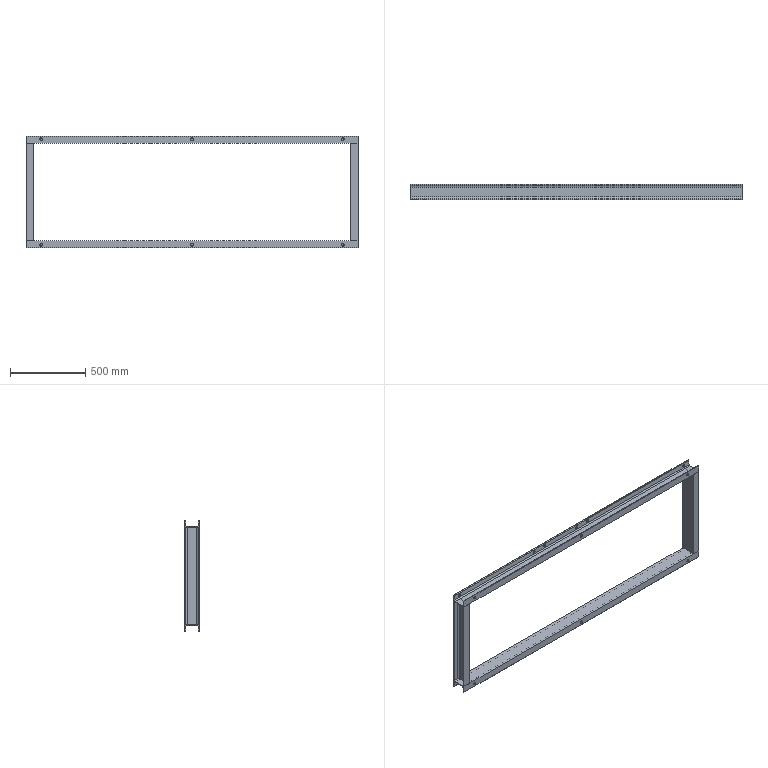Part | STEP file | MC-Base_default<by machining> | 4 solids | 92 faces | box 2202 x 100 x 740 mm | volume 7123647 mm3 | cylinder 52 | plane 40 | commonest cylinder face diameters 18 x36 8.5 x8 17 x8